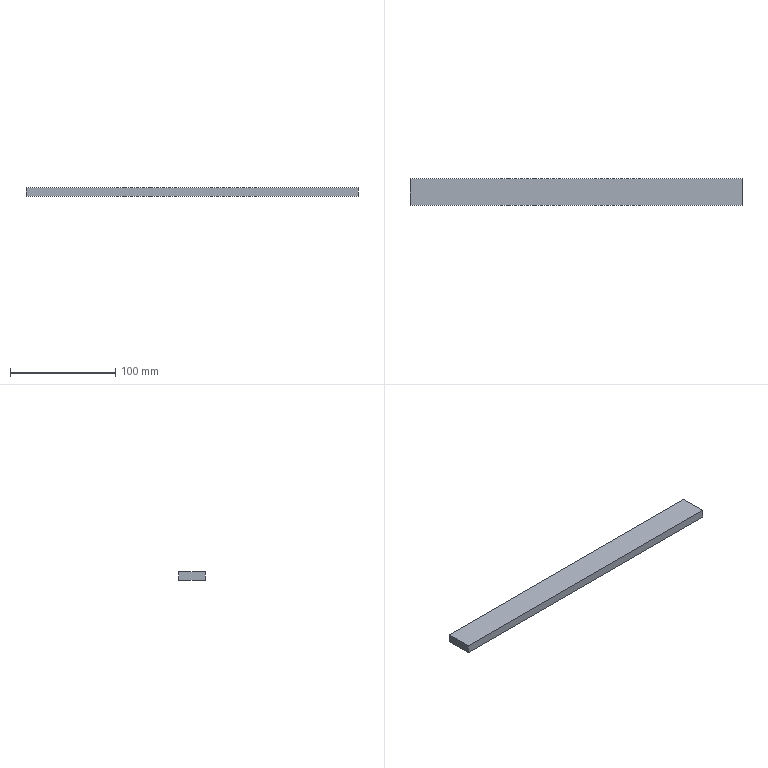Part | STEP file | 垫块1- | 1 solid | 6 faces | box 315 x 25.5 x 7.95 mm | volume 63858 mm3 | plane 6
STEP:
#1=CARTESIAN_POINT('',(190.,6.5,7.95));
#2=VERTEX_POINT('',#1);
#3=CARTESIAN_POINT('',(190.,32.,7.95));
#4=VERTEX_POINT('',#3);
#5=CARTESIAN_POINT('',(190.,32.,7.95));
#6=DIRECTION('',(0.,1.,0.));
#7=VECTOR('',#6,1000.);
#8=LINE('',#5,#7);
#9=EDGE_CURVE('',#2,#4,#8,.T.);
#10=ORIENTED_EDGE('',*,*,#9,.F.);
#11=CARTESIAN_POINT('',(190.,6.5,0.));
#12=VERTEX_POINT('',#11);
#13=CARTESIAN_POINT('',(190.,6.5,323.98));
#14=DIRECTION('',(0.,0.,-1.));
#15=VECTOR('',#14,1000.);
#16=LINE('',#13,#15);
#17=EDGE_CURVE('',#2,#12,#16,.T.);
#18=ORIENTED_EDGE('',*,*,#17,.T.);
#19=CARTESIAN_POINT('',(190.,32.,0.));
#20=VERTEX_POINT('',#19);
#21=CARTESIAN_POINT('',(190.,32.,0.));
#22=DIRECTION('',(0.,1.,0.));
#23=VECTOR('',#22,1000.);
#24=LINE('',#21,#23);
#25=EDGE_CURVE('',#12,#20,#24,.T.);
#26=ORIENTED_EDGE('',*,*,#25,.T.);
#27=CARTESIAN_POINT('',(190.,32.,323.98));
#28=DIRECTION('',(0.,0.,-1.));
#29=VECTOR('',#28,1000.);
#30=LINE('',#27,#29);
#31=EDGE_CURVE('',#4,#20,#30,.T.);
#32=ORIENTED_EDGE('',*,*,#31,.F.);
#33=EDGE_LOOP('',(#10,#18,#26,#32));
#34=FACE_OUTER_BOUND('',#33,.T.);
#35=CARTESIAN_POINT('',(190.,32.,323.98));
#36=DIRECTION('',(-1.,0.,0.));
#37=DIRECTION('',(0.,0.,1.));
#38=AXIS2_PLACEMENT_3D('',#35,#36,#37);
#39=PLANE('',#38);
#40=ADVANCED_FACE('',(#34),#39,.F.);
#41=CARTESIAN_POINT('',(-125.,32.,7.95));
#42=VERTEX_POINT('',#41);
#43=CARTESIAN_POINT('',(190.,32.,7.95));
#44=DIRECTION('',(-1.,0.,0.));
#45=VECTOR('',#44,1000.);
#46=LINE('',#43,#45);
#47=EDGE_CURVE('',#4,#42,#46,.T.);
#48=ORIENTED_EDGE('',*,*,#47,.F.);
#49=ORIENTED_EDGE('',*,*,#31,.T.);
#50=CARTESIAN_POINT('',(-125.,32.,0.));
#51=VERTEX_POINT('',#50);
#52=CARTESIAN_POINT('',(190.,32.,0.));
#53=DIRECTION('',(-1.,0.,0.));
#54=VECTOR('',#53,1000.);
#55=LINE('',#52,#54);
#56=EDGE_CURVE('',#20,#51,#55,.T.);
#57=ORIENTED_EDGE('',*,*,#56,.T.);
#58=CARTESIAN_POINT('',(-125.,32.,323.98));
#59=DIRECTION('',(0.,0.,-1.));
#60=VECTOR('',#59,1000.);
#61=LINE('',#58,#60);
#62=EDGE_CURVE('',#42,#51,#61,.T.);
#63=ORIENTED_EDGE('',*,*,#62,.F.);
#64=EDGE_LOOP('',(#48,#49,#57,#63));
#65=FACE_OUTER_BOUND('',#64,.T.);
#66=CARTESIAN_POINT('',(190.,32.,323.98));
#67=DIRECTION('',(0.,-1.,0.));
#68=DIRECTION('',(0.,0.,-1.));
#69=AXIS2_PLACEMENT_3D('',#66,#67,#68);
#70=PLANE('',#69);
#71=ADVANCED_FACE('',(#65),#70,.F.);
#72=CARTESIAN_POINT('',(-125.,6.5,7.95));
#73=VERTEX_POINT('',#72);
#74=CARTESIAN_POINT('',(-125.,32.,7.95));
#75=DIRECTION('',(0.,-1.,0.));
#76=VECTOR('',#75,1000.);
#77=LINE('',#74,#76);
#78=EDGE_CURVE('',#42,#73,#77,.T.);
#79=ORIENTED_EDGE('',*,*,#78,.F.);
#80=ORIENTED_EDGE('',*,*,#62,.T.);
#81=CARTESIAN_POINT('',(-125.,6.5,0.));
#82=VERTEX_POINT('',#81);
#83=CARTESIAN_POINT('',(-125.,32.,0.));
#84=DIRECTION('',(0.,-1.,0.));
#85=VECTOR('',#84,1000.);
#86=LINE('',#83,#85);
#87=EDGE_CURVE('',#51,#82,#86,.T.);
#88=ORIENTED_EDGE('',*,*,#87,.T.);
#89=CARTESIAN_POINT('',(-125.,6.5,323.98));
#90=DIRECTION('',(0.,0.,-1.));
#91=VECTOR('',#90,1000.);
#92=LINE('',#89,#91);
#93=EDGE_CURVE('',#73,#82,#92,.T.);
#94=ORIENTED_EDGE('',*,*,#93,.F.);
#95=EDGE_LOOP('',(#79,#80,#88,#94));
#96=FACE_OUTER_BOUND('',#95,.T.);
#97=CARTESIAN_POINT('',(-125.,32.,323.98));
#98=DIRECTION('',(1.,0.,0.));
#99=DIRECTION('',(0.,0.,-1.));
#100=AXIS2_PLACEMENT_3D('',#97,#98,#99);
#101=PLANE('',#100);
#102=ADVANCED_FACE('',(#96),#101,.F.);
#103=CARTESIAN_POINT('',(190.,6.5,7.95));
#104=DIRECTION('',(1.,0.,0.));
#105=VECTOR('',#104,1000.);
#106=LINE('',#103,#105);
#107=EDGE_CURVE('',#73,#2,#106,.T.);
#108=ORIENTED_EDGE('',*,*,#107,.F.);
#109=ORIENTED_EDGE('',*,*,#93,.T.);
#110=CARTESIAN_POINT('',(190.,6.5,0.));
#111=DIRECTION('',(1.,0.,0.));
#112=VECTOR('',#111,1000.);
#113=LINE('',#110,#112);
#114=EDGE_CURVE('',#82,#12,#113,.T.);
#115=ORIENTED_EDGE('',*,*,#114,.T.);
#116=ORIENTED_EDGE('',*,*,#17,.F.);
#117=EDGE_LOOP('',(#108,#109,#115,#116));
#118=FACE_OUTER_BOUND('',#117,.T.);
#119=CARTESIAN_POINT('',(190.,6.5,323.98));
#120=DIRECTION('',(0.,1.,0.));
#121=DIRECTION('',(0.,0.,1.));
#122=AXIS2_PLACEMENT_3D('',#119,#120,#121);
#123=PLANE('',#122);
#124=ADVANCED_FACE('',(#118),#123,.F.);
#125=ORIENTED_EDGE('',*,*,#25,.F.);
#126=ORIENTED_EDGE('',*,*,#114,.F.);
#127=ORIENTED_EDGE('',*,*,#87,.F.);
#128=ORIENTED_EDGE('',*,*,#56,.F.);
#129=EDGE_LOOP('',(#125,#126,#127,#128));
#130=FACE_OUTER_BOUND('',#129,.T.);
#131=CARTESIAN_POINT('',(0.,0.,0.));
#132=DIRECTION('',(0.,0.,-1.));
#133=DIRECTION('',(-1.,0.,0.));
#134=AXIS2_PLACEMENT_3D('',#131,#132,#133);
#135=PLANE('',#134);
#136=ADVANCED_FACE('',(#130),#135,.T.);
#137=ORIENTED_EDGE('',*,*,#107,.T.);
#138=ORIENTED_EDGE('',*,*,#9,.T.);
#139=ORIENTED_EDGE('',*,*,#47,.T.);
#140=ORIENTED_EDGE('',*,*,#78,.T.);
#141=EDGE_LOOP('',(#137,#138,#139,#140));
#142=FACE_OUTER_BOUND('',#141,.T.);
#143=CARTESIAN_POINT('',(-62.,7.25,7.95));
#144=DIRECTION('',(0.,0.,1.));
#145=DIRECTION('',(-1.,0.,0.));
#146=AXIS2_PLACEMENT_3D('',#143,#144,#145);
#147=PLANE('',#146);
#148=ADVANCED_FACE('',(#142),#147,.T.);
#149=CLOSED_SHELL('',(#40,#71,#102,#124,#136,#148));
#150=MANIFOLD_SOLID_BREP('',#149);
#151=CARTESIAN_POINT('',(0.,0.,0.));
#152=DIRECTION('',(0.,0.,1.));
#153=DIRECTION('',(1.,0.,0.));
#154=AXIS2_PLACEMENT_3D('',#151,#152,#153);
#155=(LENGTH_UNIT()NAMED_UNIT(*)SI_UNIT(.MILLI.,.METRE.));
#156=UNCERTAINTY_MEASURE_WITH_UNIT(LENGTH_MEASURE(0.00001),#155,'','');
#157=(NAMED_UNIT(*)PLANE_ANGLE_UNIT()SI_UNIT($,.RADIAN.));
#158=(NAMED_UNIT(*)SI_UNIT($,.STERADIAN.)SOLID_ANGLE_UNIT());
#159=(GEOMETRIC_REPRESENTATION_CONTEXT(3)GLOBAL_UNCERTAINTY_ASSIGNED_CONTEXT((#156))GLOBAL_UNIT_ASSIGNED_CONTEXT((#155,#157,#158))REPRESENTATION_CONTEXT('',''));
#160=ADVANCED_BREP_SHAPE_REPRESENTATION('',(#150,#154),#159);